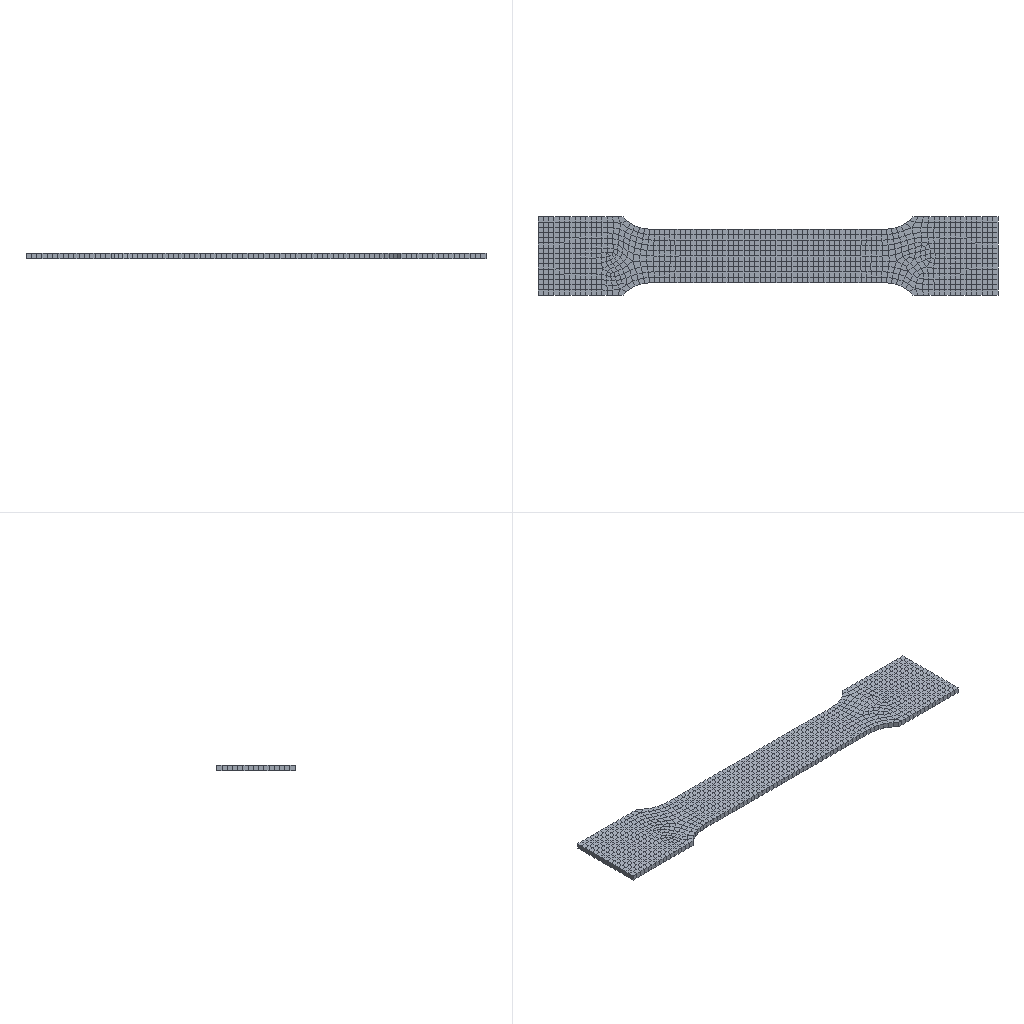Simulation study | ansys workbench
Ansys APDL input file, long lists of numbers shortened:
/batch
/config,noeldb,1     ! force off writing results to database
*get,_wallstrt,active,,time,wall
! ANSYS input file written by Workbench version 2022 R1
! File used for geometry attach: F:\ansys（分析文件汇总)\122\零件2.STEP
/title,wbnew--____ (D5)
! ****** Begin Custom Load Command Snippet ******
/COM, ACT Extensions:
/COM,     LSDYNA, 2021.1
/COM,
! ****** End   Custom Load Command Snippet ******
*DIM,_wb_ProjectScratch_dir,string,248
_wb_ProjectScratch_dir(1) = 'C:\Users\Administrator\AppData\Local\Temp\WB_Administrator_2068_2\_ProjectScratch\Scr1A2A\'
*DIM,_wb_SolverFiles_dir,string,248
_wb_SolverFiles_dir(1) = 'C:\Users\Administrator\AppData\Local\Temp\WB_Administrator_2068_2\wbnew_files\dp0\SYS-1\MECH\'
*DIM,_wb_userfiles_dir,string,248
_wb_userfiles_dir(1) = 'C:\Users\Administrator\AppData\Local\Temp\WB_Administrator_2068_2\wbnew_files\user_files\'
/com,--- Data in consistent NMM units. See Solving Units in the help system for more information.
/units,MPA
/nopr
/wb,file,start              !  signify a WB generated input file
/prep7
! Turn off shape checking because checks already performed inside WB mesher.
! See help system for more information.
SHPP,OFF,,NOWARN
/nolist
etcon,set             ! allow ANSYS to choose best KEYOP's for 180x elements, resets any applicable keyopt to MAPDL defaults
/com,*********** Nodes for the whole assembly ***********
nblock,3,,1123261
(1i9,3e20.9e3)
        1    -3.970037453E+02     2.500000000E+00    -2.970000000E+02
! (1021146 more lines like these left out)
-1
/wb,elem,start            !  set before creation of elements
/com,*********** Elements for Body 1 "__2-FreeParts|__-__1" ***********
et,1,186
keyo,1,2,1          ! set full integration on SOLID186
eblock,19,solid,,213600
(19i9)
        1        1        1        1        0        0        0        0       20        0        1        1   267675   267474   266409   211736   268074   267473   267472
! (427199 more lines like these left out)
-1
/wb,elem,end               !  done creating elements
/com,*********** Send User Defined Coordinate System(s) ***********
csys,0
toffst,273.15,  ! Temperature offset from absolute zero
/com,*********** Set Reference Temperature ***********
tref,22.
/wb,mat,start              !  starting to send materials
/com,*********** Send Materials ***********
Temperature = 'TEMP' ! Temperature
MP,DENS,1,7.85e-09,	! tonne mm^-3
MP,ALPX,1,1.2e-05,	! C^-1
MP,C,1,434000000,	! mm^2 s^-2 C^-1
MP,KXX,1,60.5,	! tonne mm s^-3 C^-1
MP,RSVX,1,0.00017,	! ohm mm
MP,EX,1,200000,	! tonne s^-2 mm^-1
MP,NUXY,1,0.3,
MP,MURX,1,10000,
/wb,mat,end                !  done sending materials
!************************* Model Summary ********************
!__2-FreeParts|__-__1,	结构钢,	matid,	1
!************************* End Model Summary ********************
! get the diagonal of the bounding box. Needed later for other things
*get,_xmin,node,,mnloc,x
*get,_ymin,node,,mnloc,y
*get,_zmin,node,,mnloc,z
*get,_xmax,node,,mxloc,x
*get,_ymax,node,,mxloc,y
*get,_zmax,node,,mxloc,z
_ASMDIAG=(_xmax-_xmin)*(_xmax-_xmin)+(_ymax-_ymin)*(_ymax-_ymin)+(_zmax-_zmin)*(_zmax-_zmin)
_ASMDIAG=SQRT(_ASMDIAG)
/wb,contact,start          !  starting to send contact
/wb,contact,end            !  done creating contacts
/golist
/wb,load,start             !  starting to send loads
/com,******* Constant Zero Displacement X *******
CMBLOCK,_DISPZEROUX,NODE,        4
(8i10)
    264937    265137    265404    265604
cmsel,s,_DISPZEROUX
d,all,ux,0
nsel,all
/com,******* Constant Zero Displacement Y *******
CMBLOCK,_DISPZEROUY,NODE,        4
(8i10)
    264937    265137    265404    265604
cmsel,s,_DISPZEROUY
d,all,uy,0
nsel,all
/com,******* Constant Zero Displacement Z *******
CMBLOCK,_DISPZEROUZ,NODE,        4
(8i10)
    264937    265137    265404    265604
cmsel,s,_DISPZEROUZ
d,all,uz,0
nsel,all
/com,*********** Define Force Using Surface Effect Elements ***********
local,12,0,0.,0.,0.,0.,0.,0.
csys,0
et,2,154
eblock,10,,,1068
(15i9)
   324137        2        2        2       12   267474   266409   267472   267473  1016024  1016023  1017882  1017883
! (1067 more lines like these left out)
-1
esel,s,type,,2
keyop,2,2,1                ! Apply load in local coordinate system
keyop,2,7,1                ! Use original area so load is constant in large deformation
esel,all
/com,*********** Define Force Using Surface Effect Elements ***********
local,13,0,0.,0.,0.,0.,0.,0.
csys,0
et,3,154
eblock,10,,,1068
(15i9)
   325205        3        3        3       13   268276   268277   264936   264937  1019289  1013274  1013273  1013276
! (1067 more lines like these left out)
-1
esel,s,type,,3
keyop,3,2,1                ! Apply load in local coordinate system
keyop,3,7,1                ! Use original area so load is constant in large deformation
esel,all
/com,*********** Define Force Using Surface Effect Elements ***********
local,14,0,0.,0.,0.,0.,0.,0.
csys,0
et,4,154
eblock,10,,,800
(15i9)
   326273        4        4        4       14   268274   267477   268272   268273  1017893  1017892  1019282  1019283
! (799 more lines like these left out)
-1
esel,s,type,,4
keyop,4,2,1                ! Apply load in local coordinate system
keyop,4,7,1                ! Use original area so load is constant in large deformation
esel,all
/com,*********** Define Force Using Surface Effect Elements ***********
local,15,0,0.,0.,0.,0.,0.,0.
csys,0
et,5,154
eblock,10,,,800
(15i9)
   327073        5        5        5       15   265405   265605   266408   265404  1014212  1014612  1014210  1014209
! (799 more lines like these left out)
-1
esel,s,type,,5
keyop,5,2,1                ! Apply load in local coordinate system
keyop,5,7,1                ! Use original area so load is constant in large deformation
esel,all
/gst,on,on
fini
*get,_numnode,node,0,count
*get,_numelem,elem,0,count
*get, _MAXELEMNUM, elem, 0, NUM, MAX
*get, _MAXNODENUM, node, 0, NUM, MAX
*get, _MAXELEMTYPE, etyp, 0, NUM, MAX
*get, _MAXREALCONST, real, 0, NUM, MAX
/go
/wb,load,end               !  done creating loads
/com,--- Number of total nodes = %_numnode%
/com,--- Number of contact elements = 3736
/com,--- Number of spring elements = 0
/com,--- Number of bearing elements = 0
/com,--- Number of solid elements = 213600
/com,--- Number of condensed parts = 0
/com,--- Number of total elements = %_numelem%
*get,_wallbsol,active,,time,wall
/com,****************************************************************************
/com,*************************    SOLUTION       ********************************
/com,****************************************************************************
/solu
antype,0                   ! static analysis
_thickRatio=  1     ! Ratio of thick parts in the model
eqsl,pcg,1e-8,,,,,,1
msave,on
cntr,print,1               ! print out contact info and also make no initial contact an error
dmpoption,emat,no             ! Don't combine emat file for DANSYS
dmpoption,esav,no             ! Don't combine esav file for DANSYS
nldiag,cont,iter           ! print out contact info each equilibrium iteration
rescontrol,,none                 ! Do not keep any restart files
/com,****************************************************
/com,******************* SOLVE FOR LS 1 OF 1 ****************
esel,s,type,,2
nsle
sfe,all,1,pres,1,-3.46944695195387e-019
sfe,all,2,pres,1,0.
sfe,all,3,pres,1,-5.00000000000038e-003
esel,s,type,,3
nsle
sfe,all,1,pres,1,-6.93889390390775e-019
sfe,all,2,pres,1,0.
sfe,all,3,pres,1,5.00000000000037e-003
esel,s,type,,4
nsle
sfe,all,1,pres,1,-1.33333333333345e-002
sfe,all,2,pres,1,0.
sfe,all,3,pres,1,1.23358110906164e-018
esel,s,type,,5
nsle
sfe,all,1,pres,1,1.33333333333344e-002
sfe,all,2,pres,1,0.
sfe,all,3,pres,1,-2.46716221812326e-018
nsel,all
esel,all
/nopr
/gopr
nsub,1,1,1
time,1.
outres,erase
outres,all,none
outres,nsol,all,
outres,rsol,all
outres,eangl,all
outres,etmp,all
outres,veng,all
outres,strs,all,
outres,epel,all,
outres,eppl,all,
outres,cont,all,
! *********** WB SOLVE COMMAND ***********
! check interactive state
*get,ANSINTER_,active,,int
*if,ANSINTER_,ne,0,then
/eof
*endif
solve
/com *************** Write FE CONNECTORS *********
CEWRITE,file,ce,,INTE
/com,****************************************************
/com,*************** FINISHED SOLVE FOR LS 1 *************
*get,_wallasol,active,,time,wall
/nopr
*get,_numnode,node,0,count
*get,_numelem,elem,0,count
*get, _MAXELEMNUM, elem, 0, NUM, MAX
*get, _MAXNODENUM, node, 0, NUM, MAX,,,INTERNAL
*get, _MAXELEMTYPE, etyp, 0, NUM, MAX
*get, _MAXREALCONST, real, 0, NUM, MAX
/gopr
*get,_PCGITER,active,,solu,cgiter
/post1
xmlo,ENCODING,ISO-8859-1
xmlo,parm
/xml,parm,xml
fini
/gopr
*get,_walldone,active,,time,wall
_preptime=(_wallbsol-_wallstrt)*3600
_solvtime=(_wallasol-_wallbsol)*3600
_posttime=(_walldone-_wallasol)*3600
_totaltim=(_walldone-_wallstrt)*3600
*get,_dlbratio,active,0,solu,dlbr
*get,_combtime,active,0,solu,comb
*get,_ssmode,active,0,solu,ssmm
*get,_ndofs,active,0,solu,ndof
*get,_sol_end_time,active,0,set,time
*if,_sol_end_time,eq,1.,then
/fclean				!clean distributed files
*endif
/com,--- Total number of nodes = %_numnode%
/com,--- Total number of elements = %_numelem%
/com,--- Element load balance ratio = %_dlbratio%
/com,--- Time to combine distributed files = %_combtime%
/com,--- Sparse memory mode = %_ssmode%
/com,--- Number of DOF = %_ndofs%
/wb,file,end               ! done with WB generated input